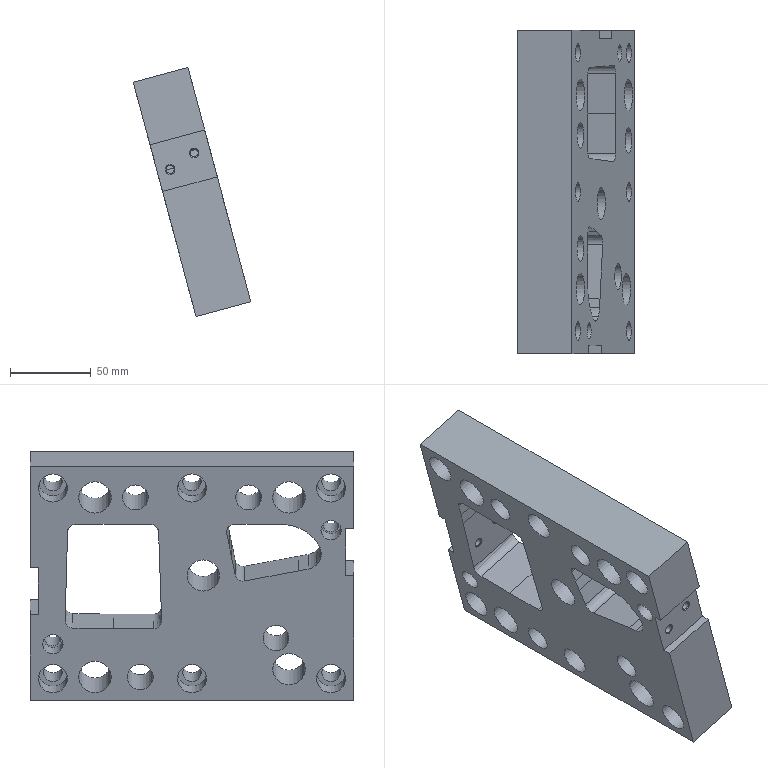Part | NX | features solid 2 | 1 solid | 103 faces | box 72.63 x 200 x 153.948 mm | volume 719460 mm3 | spline 42 | cylinder 29 | plane 28 | cone 4 | commonest cylinder face diameters 11.507 x6 18.008 x6 20 x5 5 x4 16 x4 10 x2